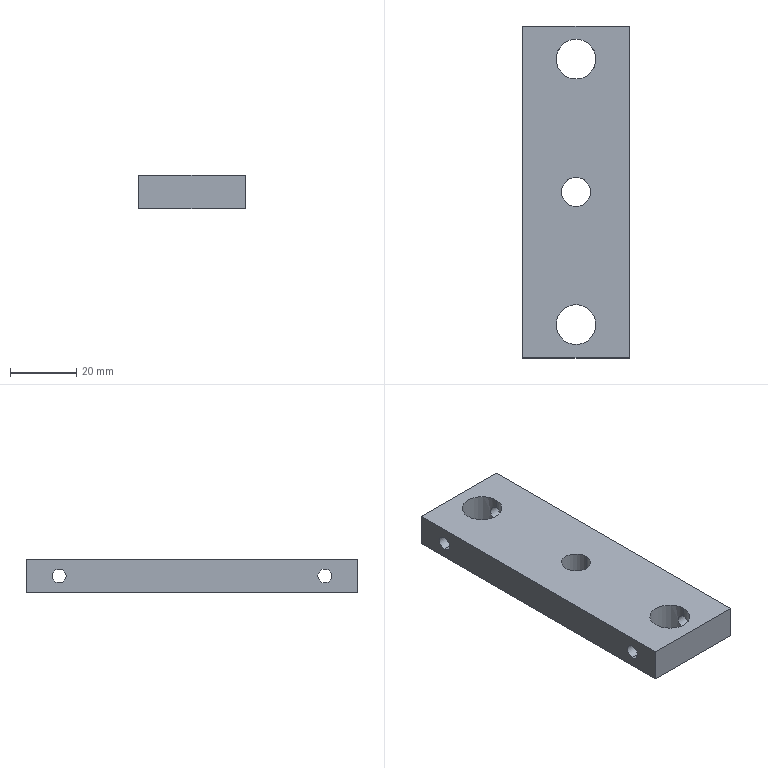Part | STEP file | X77b-01010 | 1 solid | 62 faces | box 32 x 100 x 10 mm | volume 28124 mm3 | cylinder 38 | cone 12 | plane 12 | commonest cylinder face diameters 2.5 x8 3 x8 4.2 x8 3.3 x4 4 x4 12 x4